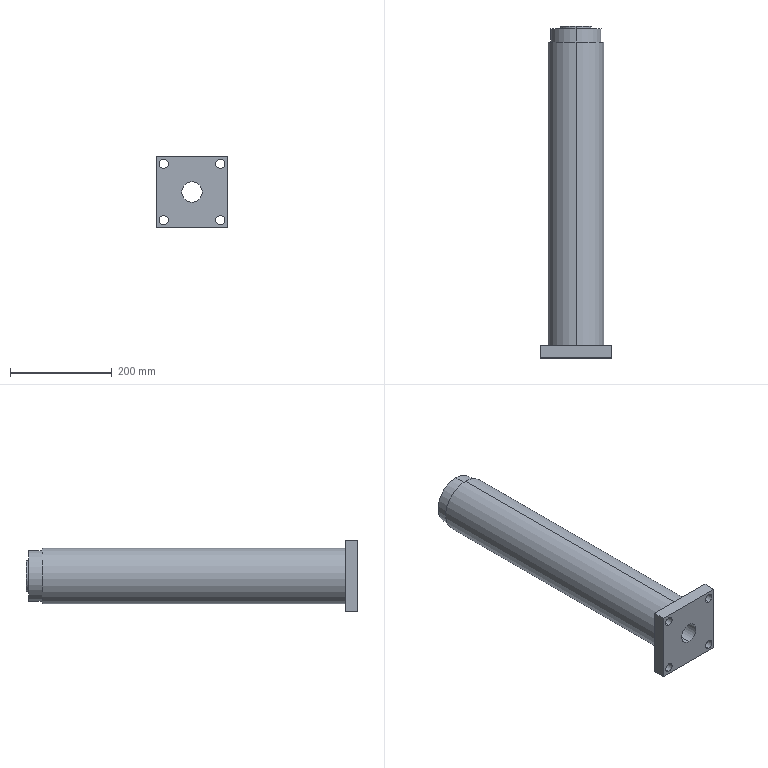Part | SolidWorks | features ICE 4, Extrusion 1 | 1 solid | 25 faces | box 140 x 652 x 140 mm | volume 5526719 mm3 | cylinder 16 | plane 9 | commonest cylinder face diameters 18 x8 40 x2 60 x2 100 x2 110 x2
STEP:
#1=CARTESIAN_POINT('',(0.,620.5,50.));
#2=VERTEX_POINT('',#1);
#3=CARTESIAN_POINT('',(0.,620.5,-50.));
#4=VERTEX_POINT('',#3);
#5=CARTESIAN_POINT('',(0.,620.5,0.));
#6=DIRECTION('',(0.,1.,0.));
#7=DIRECTION('',(0.,0.,1.));
#8=AXIS2_PLACEMENT_3D('',#5,#6,#7);
#9=CIRCLE('',#8,50.);
#10=EDGE_CURVE('',#2,#4,#9,.T.);
#11=ORIENTED_EDGE('',*,*,#10,.T.);
#12=CARTESIAN_POINT('',(0.,647.,-50.));
#13=VERTEX_POINT('',#12);
#14=CARTESIAN_POINT('',(0.,620.5,-50.));
#15=DIRECTION('',(0.,1.,0.));
#16=VECTOR('',#15,1000.);
#17=LINE('',#14,#16);
#18=EDGE_CURVE('',#4,#13,#17,.T.);
#19=ORIENTED_EDGE('',*,*,#18,.T.);
#20=CARTESIAN_POINT('',(0.,647.,50.));
#21=VERTEX_POINT('',#20);
#22=CARTESIAN_POINT('',(0.,647.,0.));
#23=DIRECTION('',(0.,1.,0.));
#24=DIRECTION('',(0.,0.,1.));
#25=AXIS2_PLACEMENT_3D('',#22,#23,#24);
#26=CIRCLE('',#25,50.);
#27=EDGE_CURVE('',#21,#13,#26,.T.);
#28=ORIENTED_EDGE('',*,*,#27,.F.);
#29=CARTESIAN_POINT('',(0.,620.5,50.));
#30=DIRECTION('',(0.,1.,0.));
#31=VECTOR('',#30,1000.);
#32=LINE('',#29,#31);
#33=EDGE_CURVE('',#2,#21,#32,.T.);
#34=ORIENTED_EDGE('',*,*,#33,.F.);
#35=EDGE_LOOP('',(#11,#19,#28,#34));
#36=FACE_OUTER_BOUND('',#35,.T.);
#37=CARTESIAN_POINT('',(0.,620.5,0.));
#38=DIRECTION('',(0.,1.,0.));
#39=DIRECTION('',(0.,0.,1.));
#40=AXIS2_PLACEMENT_3D('',#37,#38,#39);
#41=CYLINDRICAL_SURFACE('',#40,50.);
#42=ADVANCED_FACE('',(#36),#41,.T.);
#43=CARTESIAN_POINT('',(0.,647.,30.));
#44=VERTEX_POINT('',#43);
#45=CARTESIAN_POINT('',(0.,647.,-30.));
#46=VERTEX_POINT('',#45);
#47=CARTESIAN_POINT('',(0.,647.,0.));
#48=DIRECTION('',(0.,1.,0.));
#49=DIRECTION('',(0.,0.,1.));
#50=AXIS2_PLACEMENT_3D('',#47,#48,#49);
#51=CIRCLE('',#50,30.);
#52=EDGE_CURVE('',#44,#46,#51,.T.);
#53=ORIENTED_EDGE('',*,*,#52,.T.);
#54=CARTESIAN_POINT('',(0.,652.,-30.));
#55=VERTEX_POINT('',#54);
#56=CARTESIAN_POINT('',(0.,647.,-30.));
#57=DIRECTION('',(0.,1.,0.));
#58=VECTOR('',#57,1000.);
#59=LINE('',#56,#58);
#60=EDGE_CURVE('',#46,#55,#59,.T.);
#61=ORIENTED_EDGE('',*,*,#60,.T.);
#62=CARTESIAN_POINT('',(0.,652.,30.));
#63=VERTEX_POINT('',#62);
#64=CARTESIAN_POINT('',(0.,652.,0.));
#65=DIRECTION('',(0.,1.,0.));
#66=DIRECTION('',(0.,0.,1.));
#67=AXIS2_PLACEMENT_3D('',#64,#65,#66);
#68=CIRCLE('',#67,30.);
#69=EDGE_CURVE('',#63,#55,#68,.T.);
#70=ORIENTED_EDGE('',*,*,#69,.F.);
#71=CARTESIAN_POINT('',(0.,647.,30.));
#72=DIRECTION('',(0.,1.,0.));
#73=VECTOR('',#72,1000.);
#74=LINE('',#71,#73);
#75=EDGE_CURVE('',#44,#63,#74,.T.);
#76=ORIENTED_EDGE('',*,*,#75,.F.);
#77=EDGE_LOOP('',(#53,#61,#70,#76));
#78=FACE_OUTER_BOUND('',#77,.T.);
#79=CARTESIAN_POINT('',(0.,647.,0.));
#80=DIRECTION('',(0.,1.,0.));
#81=DIRECTION('',(0.,0.,1.));
#82=AXIS2_PLACEMENT_3D('',#79,#80,#81);
#83=CYLINDRICAL_SURFACE('',#82,30.);
#84=ADVANCED_FACE('',(#78),#83,.T.);
#85=CARTESIAN_POINT('',(0.,0.,-20.));
#86=VERTEX_POINT('',#85);
#87=CARTESIAN_POINT('',(0.,0.,20.));
#88=VERTEX_POINT('',#87);
#89=CARTESIAN_POINT('',(0.,0.,0.));
#90=DIRECTION('',(0.,1.,0.));
#91=DIRECTION('',(0.,0.,1.));
#92=AXIS2_PLACEMENT_3D('',#89,#90,#91);
#93=CIRCLE('',#92,20.);
#94=EDGE_CURVE('',#86,#88,#93,.T.);
#95=ORIENTED_EDGE('',*,*,#94,.F.);
#96=CARTESIAN_POINT('',(0.,652.,-20.));
#97=VERTEX_POINT('',#96);
#98=CARTESIAN_POINT('',(0.,-928.,-20.));
#99=DIRECTION('',(0.,1.,0.));
#100=VECTOR('',#99,1000.);
#101=LINE('',#98,#100);
#102=EDGE_CURVE('',#86,#97,#101,.T.);
#103=ORIENTED_EDGE('',*,*,#102,.T.);
#104=CARTESIAN_POINT('',(0.,652.,20.));
#105=VERTEX_POINT('',#104);
#106=CARTESIAN_POINT('',(0.,652.,0.));
#107=DIRECTION('',(0.,1.,0.));
#108=DIRECTION('',(0.,0.,1.));
#109=AXIS2_PLACEMENT_3D('',#106,#107,#108);
#110=CIRCLE('',#109,20.);
#111=EDGE_CURVE('',#97,#105,#110,.T.);
#112=ORIENTED_EDGE('',*,*,#111,.T.);
#113=CARTESIAN_POINT('',(0.,-928.,20.));
#114=DIRECTION('',(0.,1.,0.));
#115=VECTOR('',#114,1000.);
#116=LINE('',#113,#115);
#117=EDGE_CURVE('',#88,#105,#116,.T.);
#118=ORIENTED_EDGE('',*,*,#117,.F.);
#119=EDGE_LOOP('',(#95,#103,#112,#118));
#120=FACE_OUTER_BOUND('',#119,.T.);
#121=CARTESIAN_POINT('',(0.,-928.,0.));
#122=DIRECTION('',(0.,1.,0.));
#123=DIRECTION('',(0.,0.,1.));
#124=AXIS2_PLACEMENT_3D('',#121,#122,#123);
#125=CYLINDRICAL_SURFACE('',#124,20.);
#126=ADVANCED_FACE('',(#120),#125,.F.);
#127=CARTESIAN_POINT('',(-55.5,25.,46.5));
#128=VERTEX_POINT('',#127);
#129=CARTESIAN_POINT('',(-55.5,25.,64.5));
#130=VERTEX_POINT('',#129);
#131=CARTESIAN_POINT('',(-55.5,25.,55.5));
#132=DIRECTION('',(0.,1.,0.));
#133=DIRECTION('',(0.,0.,1.));
#134=AXIS2_PLACEMENT_3D('',#131,#132,#133);
#135=CIRCLE('',#134,9.);
#136=EDGE_CURVE('',#128,#130,#135,.T.);
#137=ORIENTED_EDGE('',*,*,#136,.T.);
#138=CARTESIAN_POINT('',(-55.5,0.,64.5));
#139=VERTEX_POINT('',#138);
#140=CARTESIAN_POINT('',(-55.5,25.,64.5));
#141=DIRECTION('',(0.,-1.,0.));
#142=VECTOR('',#141,1000.);
#143=LINE('',#140,#142);
#144=EDGE_CURVE('',#130,#139,#143,.T.);
#145=ORIENTED_EDGE('',*,*,#144,.T.);
#146=CARTESIAN_POINT('',(-55.5,0.,46.5));
#147=VERTEX_POINT('',#146);
#148=CARTESIAN_POINT('',(-55.5,0.,55.5));
#149=DIRECTION('',(0.,1.,0.));
#150=DIRECTION('',(0.,0.,1.));
#151=AXIS2_PLACEMENT_3D('',#148,#149,#150);
#152=CIRCLE('',#151,9.);
#153=EDGE_CURVE('',#147,#139,#152,.T.);
#154=ORIENTED_EDGE('',*,*,#153,.F.);
#155=CARTESIAN_POINT('',(-55.5,25.,46.5));
#156=DIRECTION('',(0.,-1.,0.));
#157=VECTOR('',#156,1000.);
#158=LINE('',#155,#157);
#159=EDGE_CURVE('',#128,#147,#158,.T.);
#160=ORIENTED_EDGE('',*,*,#159,.F.);
#161=EDGE_LOOP('',(#137,#145,#154,#160));
#162=FACE_OUTER_BOUND('',#161,.T.);
#163=CARTESIAN_POINT('',(-55.5,25.,55.5));
#164=DIRECTION('',(0.,-1.,0.));
#165=DIRECTION('',(0.,0.,-1.));
#166=AXIS2_PLACEMENT_3D('',#163,#164,#165);
#167=CYLINDRICAL_SURFACE('',#166,9.);
#168=ADVANCED_FACE('',(#162),#167,.F.);
#169=CARTESIAN_POINT('',(55.5,25.,46.5));
#170=VERTEX_POINT('',#169);
#171=CARTESIAN_POINT('',(55.5,25.,64.5));
#172=VERTEX_POINT('',#171);
#173=CARTESIAN_POINT('',(55.5,25.,55.5));
#174=DIRECTION('',(0.,1.,0.));
#175=DIRECTION('',(0.,0.,1.));
#176=AXIS2_PLACEMENT_3D('',#173,#174,#175);
#177=CIRCLE('',#176,9.);
#178=EDGE_CURVE('',#170,#172,#177,.T.);
#179=ORIENTED_EDGE('',*,*,#178,.T.);
#180=CARTESIAN_POINT('',(55.5,0.,64.5));
#181=VERTEX_POINT('',#180);
#182=CARTESIAN_POINT('',(55.5,25.,64.5));
#183=DIRECTION('',(0.,-1.,0.));
#184=VECTOR('',#183,1000.);
#185=LINE('',#182,#184);
#186=EDGE_CURVE('',#172,#181,#185,.T.);
#187=ORIENTED_EDGE('',*,*,#186,.T.);
#188=CARTESIAN_POINT('',(55.5,0.,46.5));
#189=VERTEX_POINT('',#188);
#190=CARTESIAN_POINT('',(55.5,0.,55.5));
#191=DIRECTION('',(0.,1.,0.));
#192=DIRECTION('',(0.,0.,1.));
#193=AXIS2_PLACEMENT_3D('',#190,#191,#192);
#194=CIRCLE('',#193,9.);
#195=EDGE_CURVE('',#189,#181,#194,.T.);
#196=ORIENTED_EDGE('',*,*,#195,.F.);
#197=CARTESIAN_POINT('',(55.5,25.,46.5));
#198=DIRECTION('',(0.,-1.,0.));
#199=VECTOR('',#198,1000.);
#200=LINE('',#197,#199);
#201=EDGE_CURVE('',#170,#189,#200,.T.);
#202=ORIENTED_EDGE('',*,*,#201,.F.);
#203=EDGE_LOOP('',(#179,#187,#196,#202));
#204=FACE_OUTER_BOUND('',#203,.T.);
#205=CARTESIAN_POINT('',(55.5,25.,55.5));
#206=DIRECTION('',(0.,-1.,0.));
#207=DIRECTION('',(0.,0.,-1.));
#208=AXIS2_PLACEMENT_3D('',#205,#206,#207);
#209=CYLINDRICAL_SURFACE('',#208,9.);
#210=ADVANCED_FACE('',(#204),#209,.F.);
#211=CARTESIAN_POINT('',(55.5,25.,-64.5));
#212=VERTEX_POINT('',#211);
#213=CARTESIAN_POINT('',(55.5,25.,-46.5));
#214=VERTEX_POINT('',#213);
#215=CARTESIAN_POINT('',(55.5,25.,-55.5));
#216=DIRECTION('',(0.,1.,0.));
#217=DIRECTION('',(0.,0.,1.));
#218=AXIS2_PLACEMENT_3D('',#215,#216,#217);
#219=CIRCLE('',#218,9.);
#220=EDGE_CURVE('',#212,#214,#219,.T.);
#221=ORIENTED_EDGE('',*,*,#220,.T.);
#222=CARTESIAN_POINT('',(55.5,0.,-46.5));
#223=VERTEX_POINT('',#222);
#224=CARTESIAN_POINT('',(55.5,25.,-46.5));
#225=DIRECTION('',(0.,-1.,0.));
#226=VECTOR('',#225,1000.);
#227=LINE('',#224,#226);
#228=EDGE_CURVE('',#214,#223,#227,.T.);
#229=ORIENTED_EDGE('',*,*,#228,.T.);
#230=CARTESIAN_POINT('',(55.5,0.,-64.5));
#231=VERTEX_POINT('',#230);
#232=CARTESIAN_POINT('',(55.5,0.,-55.5));
#233=DIRECTION('',(0.,1.,0.));
#234=DIRECTION('',(0.,0.,1.));
#235=AXIS2_PLACEMENT_3D('',#232,#233,#234);
#236=CIRCLE('',#235,9.);
#237=EDGE_CURVE('',#231,#223,#236,.T.);
#238=ORIENTED_EDGE('',*,*,#237,.F.);
#239=CARTESIAN_POINT('',(55.5,25.,-64.5));
#240=DIRECTION('',(0.,-1.,0.));
#241=VECTOR('',#240,1000.);
#242=LINE('',#239,#241);
#243=EDGE_CURVE('',#212,#231,#242,.T.);
#244=ORIENTED_EDGE('',*,*,#243,.F.);
#245=EDGE_LOOP('',(#221,#229,#238,#244));
#246=FACE_OUTER_BOUND('',#245,.T.);
#247=CARTESIAN_POINT('',(55.5,25.,-55.5));
#248=DIRECTION('',(0.,-1.,0.));
#249=DIRECTION('',(0.,0.,-1.));
#250=AXIS2_PLACEMENT_3D('',#247,#248,#249);
#251=CYLINDRICAL_SURFACE('',#250,9.);
#252=ADVANCED_FACE('',(#246),#251,.F.);
#253=CARTESIAN_POINT('',(-55.5,25.,-64.5));
#254=VERTEX_POINT('',#253);
#255=CARTESIAN_POINT('',(-55.5,25.,-46.5));
#256=VERTEX_POINT('',#255);
#257=CARTESIAN_POINT('',(-55.5,25.,-55.5));
#258=DIRECTION('',(0.,1.,0.));
#259=DIRECTION('',(0.,0.,1.));
#260=AXIS2_PLACEMENT_3D('',#257,#258,#259);
#261=CIRCLE('',#260,9.);
#262=EDGE_CURVE('',#254,#256,#261,.T.);
#263=ORIENTED_EDGE('',*,*,#262,.T.);
#264=CARTESIAN_POINT('',(-55.5,0.,-46.5));
#265=VERTEX_POINT('',#264);
#266=CARTESIAN_POINT('',(-55.5,25.,-46.5));
#267=DIRECTION('',(0.,-1.,0.));
#268=VECTOR('',#267,1000.);
#269=LINE('',#266,#268);
#270=EDGE_CURVE('',#256,#265,#269,.T.);
#271=ORIENTED_EDGE('',*,*,#270,.T.);
#272=CARTESIAN_POINT('',(-55.5,0.,-64.5));
#273=VERTEX_POINT('',#272);
#274=CARTESIAN_POINT('',(-55.5,0.,-55.5));
#275=DIRECTION('',(0.,1.,0.));
#276=DIRECTION('',(0.,0.,1.));
#277=AXIS2_PLACEMENT_3D('',#274,#275,#276);
#278=CIRCLE('',#277,9.);
#279=EDGE_CURVE('',#273,#265,#278,.T.);
#280=ORIENTED_EDGE('',*,*,#279,.F.);
#281=CARTESIAN_POINT('',(-55.5,25.,-64.5));
#282=DIRECTION('',(0.,-1.,0.));
#283=VECTOR('',#282,1000.);
#284=LINE('',#281,#283);
#285=EDGE_CURVE('',#254,#273,#284,.T.);
#286=ORIENTED_EDGE('',*,*,#285,.F.);
#287=EDGE_LOOP('',(#263,#271,#280,#286));
#288=FACE_OUTER_BOUND('',#287,.T.);
#289=CARTESIAN_POINT('',(-55.5,25.,-55.5));
#290=DIRECTION('',(0.,-1.,0.));
#291=DIRECTION('',(0.,0.,-1.));
#292=AXIS2_PLACEMENT_3D('',#289,#290,#291);
#293=CYLINDRICAL_SURFACE('',#292,9.);
#294=ADVANCED_FACE('',(#288),#293,.F.);
#295=CARTESIAN_POINT('',(0.,620.5,55.));
#296=VERTEX_POINT('',#295);
#297=CARTESIAN_POINT('',(0.,620.5,-55.));
#298=VERTEX_POINT('',#297);
#299=CARTESIAN_POINT('',(0.,620.5,0.));
#300=DIRECTION('',(0.,1.,0.));
#301=DIRECTION('',(0.,0.,1.));
#302=AXIS2_PLACEMENT_3D('',#299,#300,#301);
#303=CIRCLE('',#302,55.);
#304=EDGE_CURVE('',#296,#298,#303,.T.);
#305=ORIENTED_EDGE('',*,*,#304,.F.);
#306=CARTESIAN_POINT('',(0.,25.,55.));
#307=VERTEX_POINT('',#306);
#308=CARTESIAN_POINT('',(0.,652.,55.));
#309=DIRECTION('',(0.,-1.,0.));
#310=VECTOR('',#309,1000.);
#311=LINE('',#308,#310);
#312=EDGE_CURVE('',#296,#307,#311,.T.);
#313=ORIENTED_EDGE('',*,*,#312,.T.);
#314=CARTESIAN_POINT('',(0.,25.,-55.));
#315=VERTEX_POINT('',#314);
#316=CARTESIAN_POINT('',(0.,25.,0.));
#317=DIRECTION('',(0.,-1.,0.));
#318=DIRECTION('',(0.,0.,1.));
#319=AXIS2_PLACEMENT_3D('',#316,#317,#318);
#320=CIRCLE('',#319,55.);
#321=EDGE_CURVE('',#315,#307,#320,.T.);
#322=ORIENTED_EDGE('',*,*,#321,.F.);
#323=CARTESIAN_POINT('',(0.,652.,-55.));
#324=DIRECTION('',(0.,-1.,0.));
#325=VECTOR('',#324,1000.);
#326=LINE('',#323,#325);
#327=EDGE_CURVE('',#298,#315,#326,.T.);
#328=ORIENTED_EDGE('',*,*,#327,.F.);
#329=EDGE_LOOP('',(#305,#313,#322,#328));
#330=FACE_OUTER_BOUND('',#329,.T.);
#331=CARTESIAN_POINT('',(0.,652.,0.));
#332=DIRECTION('',(0.,-1.,0.));
#333=DIRECTION('',(0.,0.,-1.));
#334=AXIS2_PLACEMENT_3D('',#331,#332,#333);
#335=CYLINDRICAL_SURFACE('',#334,55.);
#336=ADVANCED_FACE('',(#330),#335,.T.);
#337=ORIENTED_EDGE('',*,*,#312,.F.);
#338=CARTESIAN_POINT('',(0.,620.5,0.));
#339=DIRECTION('',(0.,1.,0.));
#340=DIRECTION('',(0.,0.,1.));
#341=AXIS2_PLACEMENT_3D('',#338,#339,#340);
#342=CIRCLE('',#341,55.);
#343=EDGE_CURVE('',#298,#296,#342,.T.);
#344=ORIENTED_EDGE('',*,*,#343,.F.);
#345=ORIENTED_EDGE('',*,*,#327,.T.);
#346=CARTESIAN_POINT('',(0.,25.,0.));
#347=DIRECTION('',(0.,-1.,0.));
#348=DIRECTION('',(0.,0.,1.));
#349=AXIS2_PLACEMENT_3D('',#346,#347,#348);
#350=CIRCLE('',#349,55.);
#351=EDGE_CURVE('',#307,#315,#350,.T.);
#352=ORIENTED_EDGE('',*,*,#351,.F.);
#353=EDGE_LOOP('',(#337,#344,#345,#352));
#354=FACE_OUTER_BOUND('',#353,.T.);
#355=CARTESIAN_POINT('',(0.,652.,0.));
#356=DIRECTION('',(0.,-1.,0.));
#357=DIRECTION('',(0.,0.,-1.));
#358=AXIS2_PLACEMENT_3D('',#355,#356,#357);
#359=CYLINDRICAL_SURFACE('',#358,55.);
#360=ADVANCED_FACE('',(#354),#359,.T.);
#361=ORIENTED_EDGE('',*,*,#52,.F.);
#362=CARTESIAN_POINT('',(0.,647.,0.));
#363=DIRECTION('',(0.,1.,0.));
#364=DIRECTION('',(0.,0.,1.));
#365=AXIS2_PLACEMENT_3D('',#362,#363,#364);
#366=CIRCLE('',#365,30.);
#367=EDGE_CURVE('',#46,#44,#366,.T.);
#368=ORIENTED_EDGE('',*,*,#367,.F.);
#369=EDGE_LOOP('',(#361,#368));
#370=FACE_BOUND('',#369,.T.);
#371=ORIENTED_EDGE('',*,*,#27,.T.);
#372=CARTESIAN_POINT('',(0.,647.,0.));
#373=DIRECTION('',(0.,1.,0.));
#374=DIRECTION('',(0.,0.,1.));
#375=AXIS2_PLACEMENT_3D('',#372,#373,#374);
#376=CIRCLE('',#375,50.);
#377=EDGE_CURVE('',#13,#21,#376,.T.);
#378=ORIENTED_EDGE('',*,*,#377,.T.);
#379=EDGE_LOOP('',(#371,#378));
#380=FACE_OUTER_BOUND('',#379,.T.);
#381=CARTESIAN_POINT('',(0.,647.,0.));
#382=DIRECTION('',(0.,1.,0.));
#383=DIRECTION('',(0.,0.,1.));
#384=AXIS2_PLACEMENT_3D('',#381,#382,#383);
#385=PLANE('',#384);
#386=ADVANCED_FACE('',(#370,#380),#385,.T.);
#387=CARTESIAN_POINT('',(0.,652.,0.));
#388=DIRECTION('',(0.,1.,0.));
#389=DIRECTION('',(0.,0.,1.));
#390=AXIS2_PLACEMENT_3D('',#387,#388,#389);
#391=CIRCLE('',#390,20.);
#392=EDGE_CURVE('',#105,#97,#391,.T.);
#393=ORIENTED_EDGE('',*,*,#392,.F.);
#394=ORIENTED_EDGE('',*,*,#111,.F.);
#395=EDGE_LOOP('',(#393,#394));
#396=FACE_BOUND('',#395,.T.);
#397=ORIENTED_EDGE('',*,*,#69,.T.);
#398=CARTESIAN_POINT('',(0.,652.,0.));
#399=DIRECTION('',(0.,1.,0.));
#400=DIRECTION('',(0.,0.,1.));
#401=AXIS2_PLACEMENT_3D('',#398,#399,#400);
#402=CIRCLE('',#401,30.);
#403=EDGE_CURVE('',#55,#63,#402,.T.);
#404=ORIENTED_EDGE('',*,*,#403,.T.);
#405=EDGE_LOOP('',(#397,#404));
#406=FACE_OUTER_BOUND('',#405,.T.);
#407=CARTESIAN_POINT('',(0.,652.,0.));
#408=DIRECTION('',(0.,1.,0.));
#409=DIRECTION('',(0.,0.,1.));
#410=AXIS2_PLACEMENT_3D('',#407,#408,#409);
#411=PLANE('',#410);
#412=ADVANCED_FACE('',(#396,#406),#411,.T.);
#413=ORIENTED_EDGE('',*,*,#321,.T.);
#414=ORIENTED_EDGE('',*,*,#351,.T.);
#415=EDGE_LOOP('',(#413,#414));
#416=FACE_BOUND('',#415,.T.);
#417=ORIENTED_EDGE('',*,*,#178,.F.);
#418=CARTESIAN_POINT('',(55.5,25.,55.5));
#419=DIRECTION('',(0.,1.,0.));
#420=DIRECTION('',(0.,0.,1.));
#421=AXIS2_PLACEMENT_3D('',#418,#419,#420);
#422=CIRCLE('',#421,9.);
#423=EDGE_CURVE('',#172,#170,#422,.T.);
#424=ORIENTED_EDGE('',*,*,#423,.F.);
#425=EDGE_LOOP('',(#417,#424));
#426=FACE_BOUND('',#425,.T.);
#427=ORIENTED_EDGE('',*,*,#262,.F.);
#428=CARTESIAN_POINT('',(-55.5,25.,-55.5));
#429=DIRECTION('',(0.,1.,0.));
#430=DIRECTION('',(0.,0.,1.));
#431=AXIS2_PLACEMENT_3D('',#428,#429,#430);
#432=CIRCLE('',#431,9.);
#433=EDGE_CURVE('',#256,#254,#432,.T.);
#434=ORIENTED_EDGE('',*,*,#433,.F.);
#435=EDGE_LOOP('',(#427,#434));
#436=FACE_BOUND('',#435,.T.);
#437=CARTESIAN_POINT('',(-70.,25.,-70.));
#438=VERTEX_POINT('',#437);
#439=CARTESIAN_POINT('',(-70.,25.,70.));
#440=VERTEX_POINT('',#439);
#441=CARTESIAN_POINT('',(-70.,25.,70.));
#442=DIRECTION('',(0.,0.,1.));
#443=VECTOR('',#442,1000.);
#444=LINE('',#441,#443);
#445=EDGE_CURVE('',#438,#440,#444,.T.);
#446=ORIENTED_EDGE('',*,*,#445,.T.);
#447=CARTESIAN_POINT('',(70.,25.,70.));
#448=VERTEX_POINT('',#447);
#449=CARTESIAN_POINT('',(70.,25.,70.));
#450=DIRECTION('',(1.,0.,0.));
#451=VECTOR('',#450,1000.);
#452=LINE('',#449,#451);
#453=EDGE_CURVE('',#440,#448,#452,.T.);
#454=ORIENTED_EDGE('',*,*,#453,.T.);
#455=CARTESIAN_POINT('',(70.,25.,-70.));
#456=VERTEX_POINT('',#455);
#457=CARTESIAN_POINT('',(70.,25.,70.));
#458=DIRECTION('',(0.,0.,-1.));
#459=VECTOR('',#458,1000.);
#460=LINE('',#457,#459);
#461=EDGE_CURVE('',#448,#456,#460,.T.);
#462=ORIENTED_EDGE('',*,*,#461,.T.);
#463=CARTESIAN_POINT('',(70.,25.,-70.));
#464=DIRECTION('',(-1.,0.,0.));
#465=VECTOR('',#464,1000.);
#466=LINE('',#463,#465);
#467=EDGE_CURVE('',#456,#438,#466,.T.);
#468=ORIENTED_EDGE('',*,*,#467,.T.);
#469=EDGE_LOOP('',(#446,#454,#462,#468));
#470=FACE_OUTER_BOUND('',#469,.T.);
#471=ORIENTED_EDGE('',*,*,#220,.F.);
#472=CARTESIAN_POINT('',(55.5,25.,-55.5));
#473=DIRECTION('',(0.,1.,0.));
#474=DIRECTION('',(0.,0.,1.));
#475=AXIS2_PLACEMENT_3D('',#472,#473,#474);
#476=CIRCLE('',#475,9.);
#477=EDGE_CURVE('',#214,#212,#476,.T.);
#478=ORIENTED_EDGE('',*,*,#477,.F.);
#479=EDGE_LOOP('',(#471,#478));
#480=FACE_BOUND('',#479,.T.);
#481=ORIENTED_EDGE('',*,*,#136,.F.);
#482=CARTESIAN_POINT('',(-55.5,25.,55.5));
#483=DIRECTION('',(0.,1.,0.));
#484=DIRECTION('',(0.,0.,1.));
#485=AXIS2_PLACEMENT_3D('',#482,#483,#484);
#486=CIRCLE('',#485,9.);
#487=EDGE_CURVE('',#130,#128,#486,.T.);
#488=ORIENTED_EDGE('',*,*,#487,.F.);
#489=EDGE_LOOP('',(#481,#488));
#490=FACE_BOUND('',#489,.T.);
#491=CARTESIAN_POINT('',(0.,25.,0.));
#492=DIRECTION('',(0.,1.,0.));
#493=DIRECTION('',(0.,0.,1.));
#494=AXIS2_PLACEMENT_3D('',#491,#492,#493);
#495=PLANE('',#494);
#496=ADVANCED_FACE('',(#416,#426,#436,#470,#480,#490),#495,.T.);
#497=CARTESIAN_POINT('',(0.,0.,0.));
#498=DIRECTION('',(0.,1.,0.));
#499=DIRECTION('',(0.,0.,1.));
#500=AXIS2_PLACEMENT_3D('',#497,#498,#499);
#501=CIRCLE('',#500,20.);
#502=EDGE_CURVE('',#88,#86,#501,.T.);
#503=ORIENTED_EDGE('',*,*,#502,.T.);
#504=ORIENTED_EDGE('',*,*,#94,.T.);
#505=EDGE_LOOP('',(#503,#504));
#506=FACE_BOUND('',#505,.T.);
#507=CARTESIAN_POINT('',(-70.,0.,-70.));
#508=VERTEX_POINT('',#507);
#509=CARTESIAN_POINT('',(-70.,0.,70.));
#510=VERTEX_POINT('',#509);
#511=CARTESIAN_POINT('',(-70.,0.,70.));
#512=DIRECTION('',(0.,0.,1.));
#513=VECTOR('',#512,1000.);
#514=LINE('',#511,#513);
#515=EDGE_CURVE('',#508,#510,#514,.T.);
#516=ORIENTED_EDGE('',*,*,#515,.F.);
#517=CARTESIAN_POINT('',(70.,0.,-70.));
#518=VERTEX_POINT('',#517);
#519=CARTESIAN_POINT('',(70.,0.,-70.));
#520=DIRECTION('',(-1.,0.,0.));
#521=VECTOR('',#520,1000.);
#522=LINE('',#519,#521);
#523=EDGE_CURVE('',#518,#508,#522,.T.);
#524=ORIENTED_EDGE('',*,*,#523,.F.);
#525=CARTESIAN_POINT('',(70.,0.,70.));
#526=VERTEX_POINT('',#525);
#527=CARTESIAN_POINT('',(70.,0.,70.));
#528=DIRECTION('',(0.,0.,-1.));
#529=VECTOR('',#528,1000.);
#530=LINE('',#527,#529);
#531=EDGE_CURVE('',#526,#518,#530,.T.);
#532=ORIENTED_EDGE('',*,*,#531,.F.);
#533=CARTESIAN_POINT('',(70.,0.,70.));
#534=DIRECTION('',(1.,0.,0.));
#535=VECTOR('',#534,1000.);
#536=LINE('',#533,#535);
#537=EDGE_CURVE('',#510,#526,#536,.T.);
#538=ORIENTED_EDGE('',*,*,#537,.F.);
#539=EDGE_LOOP('',(#516,#524,#532,#538));
#540=FACE_OUTER_BOUND('',#539,.T.);
#541=ORIENTED_EDGE('',*,*,#279,.T.);
#542=CARTESIAN_POINT('',(-55.5,0.,-55.5));
#543=DIRECTION('',(0.,1.,0.));
#544=DIRECTION('',(0.,0.,1.));
#545=AXIS2_PLACEMENT_3D('',#542,#543,#544);
#546=CIRCLE('',#545,9.);
#547=EDGE_CURVE('',#265,#273,#546,.T.);
#548=ORIENTED_EDGE('',*,*,#547,.T.);
#549=EDGE_LOOP('',(#541,#548));
#550=FACE_BOUND('',#549,.T.);
#551=ORIENTED_EDGE('',*,*,#237,.T.);
#552=CARTESIAN_POINT('',(55.5,0.,-55.5));
#553=DIRECTION('',(0.,1.,0.));
#554=DIRECTION('',(0.,0.,1.));
#555=AXIS2_PLACEMENT_3D('',#552,#553,#554);
#556=CIRCLE('',#555,9.);
#557=EDGE_CURVE('',#223,#231,#556,.T.);
#558=ORIENTED_EDGE('',*,*,#557,.T.);
#559=EDGE_LOOP('',(#551,#558));
#560=FACE_BOUND('',#559,.T.);
#561=ORIENTED_EDGE('',*,*,#195,.T.);
#562=CARTESIAN_POINT('',(55.5,0.,55.5));
#563=DIRECTION('',(0.,1.,0.));
#564=DIRECTION('',(0.,0.,1.));
#565=AXIS2_PLACEMENT_3D('',#562,#563,#564);
#566=CIRCLE('',#565,9.);
#567=EDGE_CURVE('',#181,#189,#566,.T.);
#568=ORIENTED_EDGE('',*,*,#567,.T.);
#569=EDGE_LOOP('',(#561,#568));
#570=FACE_BOUND('',#569,.T.);
#571=ORIENTED_EDGE('',*,*,#153,.T.);
#572=CARTESIAN_POINT('',(-55.5,0.,55.5));
#573=DIRECTION('',(0.,1.,0.));
#574=DIRECTION('',(0.,0.,1.));
#575=AXIS2_PLACEMENT_3D('',#572,#573,#574);
#576=CIRCLE('',#575,9.);
#577=EDGE_CURVE('',#139,#147,#576,.T.);
#578=ORIENTED_EDGE('',*,*,#577,.T.);
#579=EDGE_LOOP('',(#571,#578));
#580=FACE_BOUND('',#579,.T.);
#581=CARTESIAN_POINT('',(0.,0.,0.));
#582=DIRECTION('',(0.,1.,0.));
#583=DIRECTION('',(0.,0.,1.));
#584=AXIS2_PLACEMENT_3D('',#581,#582,#583);
#585=PLANE('',#584);
#586=ADVANCED_FACE('',(#506,#540,#550,#560,#570,#580),#585,.F.);
#587=ORIENTED_EDGE('',*,*,#515,.T.);
#588=CARTESIAN_POINT('',(-70.,25.,70.));
#589=DIRECTION('',(0.,-1.,0.));
#590=VECTOR('',#589,1000.);
#591=LINE('',#588,#590);
#592=EDGE_CURVE('',#440,#510,#591,.T.);
#593=ORIENTED_EDGE('',*,*,#592,.F.);
#594=ORIENTED_EDGE('',*,*,#445,.F.);
#595=CARTESIAN_POINT('',(-70.,25.,-70.));
#596=DIRECTION('',(0.,-1.,0.));
#597=VECTOR('',#596,1000.);
#598=LINE('',#595,#597);
#599=EDGE_CURVE('',#438,#508,#598,.T.);
#600=ORIENTED_EDGE('',*,*,#599,.T.);
#601=EDGE_LOOP('',(#587,#593,#594,#600));
#602=FACE_OUTER_BOUND('',#601,.T.);
#603=CARTESIAN_POINT('',(-70.,25.,70.));
#604=DIRECTION('',(1.,0.,0.));
#605=DIRECTION('',(0.,0.,-1.));
#606=AXIS2_PLACEMENT_3D('',#603,#604,#605);
#607=PLANE('',#606);
#608=ADVANCED_FACE('',(#602),#607,.F.);
#609=ORIENTED_EDGE('',*,*,#537,.T.);
#610=CARTESIAN_POINT('',(70.,25.,70.));
#611=DIRECTION('',(0.,-1.,0.));
#612=VECTOR('',#611,1000.);
#613=LINE('',#610,#612);
#614=EDGE_CURVE('',#448,#526,#613,.T.);
#615=ORIENTED_EDGE('',*,*,#614,.F.);
#616=ORIENTED_EDGE('',*,*,#453,.F.);
#617=ORIENTED_EDGE('',*,*,#592,.T.);
#618=EDGE_LOOP('',(#609,#615,#616,#617));
#619=FACE_OUTER_BOUND('',#618,.T.);
#620=CARTESIAN_POINT('',(70.,25.,70.));
#621=DIRECTION('',(0.,0.,-1.));
#622=DIRECTION('',(-1.,0.,0.));
#623=AXIS2_PLACEMENT_3D('',#620,#621,#622);
#624=PLANE('',#623);
#625=ADVANCED_FACE('',(#619),#624,.F.);
#626=ORIENTED_EDGE('',*,*,#531,.T.);
#627=CARTESIAN_POINT('',(70.,25.,-70.));
#628=DIRECTION('',(0.,-1.,0.));
#629=VECTOR('',#628,1000.);
#630=LINE('',#627,#629);
#631=EDGE_CURVE('',#456,#518,#630,.T.);
#632=ORIENTED_EDGE('',*,*,#631,.F.);
#633=ORIENTED_EDGE('',*,*,#461,.F.);
#634=ORIENTED_EDGE('',*,*,#614,.T.);
#635=EDGE_LOOP('',(#626,#632,#633,#634));
#636=FACE_OUTER_BOUND('',#635,.T.);
#637=CARTESIAN_POINT('',(70.,25.,70.));
#638=DIRECTION('',(-1.,0.,0.));
#639=DIRECTION('',(0.,0.,1.));
#640=AXIS2_PLACEMENT_3D('',#637,#638,#639);
#641=PLANE('',#640);
#642=ADVANCED_FACE('',(#636),#641,.F.);
#643=ORIENTED_EDGE('',*,*,#523,.T.);
#644=ORIENTED_EDGE('',*,*,#599,.F.);
#645=ORIENTED_EDGE('',*,*,#467,.F.);
#646=ORIENTED_EDGE('',*,*,#631,.T.);
#647=EDGE_LOOP('',(#643,#644,#645,#646));
#648=FACE_OUTER_BOUND('',#647,.T.);
#649=CARTESIAN_POINT('',(70.,25.,-70.));
#650=DIRECTION('',(0.,0.,1.));
#651=DIRECTION('',(1.,0.,0.));
#652=AXIS2_PLACEMENT_3D('',#649,#650,#651);
#653=PLANE('',#652);
#654=ADVANCED_FACE('',(#648),#653,.F.);
#655=ORIENTED_EDGE('',*,*,#270,.F.);
#656=ORIENTED_EDGE('',*,*,#433,.T.);
#657=ORIENTED_EDGE('',*,*,#285,.T.);
#658=ORIENTED_EDGE('',*,*,#547,.F.);
#659=EDGE_LOOP('',(#655,#656,#657,#658));
#660=FACE_OUTER_BOUND('',#659,.T.);
#661=CARTESIAN_POINT('',(-55.5,25.,-55.5));
#662=DIRECTION('',(0.,-1.,0.));
#663=DIRECTION('',(0.,0.,-1.));
#664=AXIS2_PLACEMENT_3D('',#661,#662,#663);
#665=CYLINDRICAL_SURFACE('',#664,9.);
#666=ADVANCED_FACE('',(#660),#665,.F.);
#667=ORIENTED_EDGE('',*,*,#228,.F.);
#668=ORIENTED_EDGE('',*,*,#477,.T.);
#669=ORIENTED_EDGE('',*,*,#243,.T.);
#670=ORIENTED_EDGE('',*,*,#557,.F.);
#671=EDGE_LOOP('',(#667,#668,#669,#670));
#672=FACE_OUTER_BOUND('',#671,.T.);
#673=CARTESIAN_POINT('',(55.5,25.,-55.5));
#674=DIRECTION('',(0.,-1.,0.));
#675=DIRECTION('',(0.,0.,-1.));
#676=AXIS2_PLACEMENT_3D('',#673,#674,#675);
#677=CYLINDRICAL_SURFACE('',#676,9.);
#678=ADVANCED_FACE('',(#672),#677,.F.);
#679=ORIENTED_EDGE('',*,*,#186,.F.);
#680=ORIENTED_EDGE('',*,*,#423,.T.);
#681=ORIENTED_EDGE('',*,*,#201,.T.);
#682=ORIENTED_EDGE('',*,*,#567,.F.);
#683=EDGE_LOOP('',(#679,#680,#681,#682));
#684=FACE_OUTER_BOUND('',#683,.T.);
#685=CARTESIAN_POINT('',(55.5,25.,55.5));
#686=DIRECTION('',(0.,-1.,0.));
#687=DIRECTION('',(0.,0.,-1.));
#688=AXIS2_PLACEMENT_3D('',#685,#686,#687);
#689=CYLINDRICAL_SURFACE('',#688,9.);
#690=ADVANCED_FACE('',(#684),#689,.F.);
#691=ORIENTED_EDGE('',*,*,#144,.F.);
#692=ORIENTED_EDGE('',*,*,#487,.T.);
#693=ORIENTED_EDGE('',*,*,#159,.T.);
#694=ORIENTED_EDGE('',*,*,#577,.F.);
#695=EDGE_LOOP('',(#691,#692,#693,#694));
#696=FACE_OUTER_BOUND('',#695,.T.);
#697=CARTESIAN_POINT('',(-55.5,25.,55.5));
#698=DIRECTION('',(0.,-1.,0.));
#699=DIRECTION('',(0.,0.,-1.));
#700=AXIS2_PLACEMENT_3D('',#697,#698,#699);
#701=CYLINDRICAL_SURFACE('',#700,9.);
#702=ADVANCED_FACE('',(#696),#701,.F.);
#703=ORIENTED_EDGE('',*,*,#102,.F.);
#704=ORIENTED_EDGE('',*,*,#502,.F.);
#705=ORIENTED_EDGE('',*,*,#117,.T.);
#706=ORIENTED_EDGE('',*,*,#392,.T.);
#707=EDGE_LOOP('',(#703,#704,#705,#706));
#708=FACE_OUTER_BOUND('',#707,.T.);
#709=CARTESIAN_POINT('',(0.,-928.,0.));
#710=DIRECTION('',(0.,1.,0.));
#711=DIRECTION('',(0.,0.,1.));
#712=AXIS2_PLACEMENT_3D('',#709,#710,#711);
#713=CYLINDRICAL_SURFACE('',#712,20.);
#714=ADVANCED_FACE('',(#708),#713,.F.);
#715=ORIENTED_EDGE('',*,*,#60,.F.);
#716=ORIENTED_EDGE('',*,*,#367,.T.);
#717=ORIENTED_EDGE('',*,*,#75,.T.);
#718=ORIENTED_EDGE('',*,*,#403,.F.);
#719=EDGE_LOOP('',(#715,#716,#717,#718));
#720=FACE_OUTER_BOUND('',#719,.T.);
#721=CARTESIAN_POINT('',(0.,647.,0.));
#722=DIRECTION('',(0.,1.,0.));
#723=DIRECTION('',(0.,0.,1.));
#724=AXIS2_PLACEMENT_3D('',#721,#722,#723);
#725=CYLINDRICAL_SURFACE('',#724,30.);
#726=ADVANCED_FACE('',(#720),#725,.T.);
#727=ORIENTED_EDGE('',*,*,#10,.F.);
#728=CARTESIAN_POINT('',(0.,620.5,0.));
#729=DIRECTION('',(0.,1.,0.));
#730=DIRECTION('',(0.,0.,1.));
#731=AXIS2_PLACEMENT_3D('',#728,#729,#730);
#732=CIRCLE('',#731,50.);
#733=EDGE_CURVE('',#4,#2,#732,.T.);
#734=ORIENTED_EDGE('',*,*,#733,.F.);
#735=EDGE_LOOP('',(#727,#734));
#736=FACE_BOUND('',#735,.T.);
#737=ORIENTED_EDGE('',*,*,#343,.T.);
#738=ORIENTED_EDGE('',*,*,#304,.T.);
#739=EDGE_LOOP('',(#737,#738));
#740=FACE_OUTER_BOUND('',#739,.T.);
#741=CARTESIAN_POINT('',(0.,620.5,0.));
#742=DIRECTION('',(0.,1.,0.));
#743=DIRECTION('',(0.,0.,1.));
#744=AXIS2_PLACEMENT_3D('',#741,#742,#743);
#745=PLANE('',#744);
#746=ADVANCED_FACE('',(#736,#740),#745,.T.);
#747=ORIENTED_EDGE('',*,*,#18,.F.);
#748=ORIENTED_EDGE('',*,*,#733,.T.);
#749=ORIENTED_EDGE('',*,*,#33,.T.);
#750=ORIENTED_EDGE('',*,*,#377,.F.);
#751=EDGE_LOOP('',(#747,#748,#749,#750));
#752=FACE_OUTER_BOUND('',#751,.T.);
#753=CARTESIAN_POINT('',(0.,620.5,0.));
#754=DIRECTION('',(0.,1.,0.));
#755=DIRECTION('',(0.,0.,1.));
#756=AXIS2_PLACEMENT_3D('',#753,#754,#755);
#757=CYLINDRICAL_SURFACE('',#756,50.);
#758=ADVANCED_FACE('',(#752),#757,.T.);
#759=CLOSED_SHELL('',(#42,#84,#126,#168,#210,#252,#294,#336,#360,#386,#412,#496,#586,#608,#625,#642,#654,#666,#678,#690,#702,#714,#726,#746,#758));
#760=MANIFOLD_SOLID_BREP('',#759);
#761=CARTESIAN_POINT('',(0.,0.,0.));
#762=DIRECTION('',(0.,0.,1.));
#763=DIRECTION('',(1.,0.,0.));
#764=AXIS2_PLACEMENT_3D('',#761,#762,#763);
#765=(LENGTH_UNIT()NAMED_UNIT(*)SI_UNIT(.MILLI.,.METRE.));
#766=UNCERTAINTY_MEASURE_WITH_UNIT(LENGTH_MEASURE(0.00001),#765,'','');
#767=(NAMED_UNIT(*)PLANE_ANGLE_UNIT()SI_UNIT($,.RADIAN.));
#768=(NAMED_UNIT(*)SI_UNIT($,.STERADIAN.)SOLID_ANGLE_UNIT());
#769=(GEOMETRIC_REPRESENTATION_CONTEXT(3)GLOBAL_UNCERTAINTY_ASSIGNED_CONTEXT((#766))GLOBAL_UNIT_ASSIGNED_CONTEXT((#765,#767,#768))REPRESENTATION_CONTEXT('',''));
#770=ADVANCED_BREP_SHAPE_REPRESENTATION('',(#760,#764),#769);